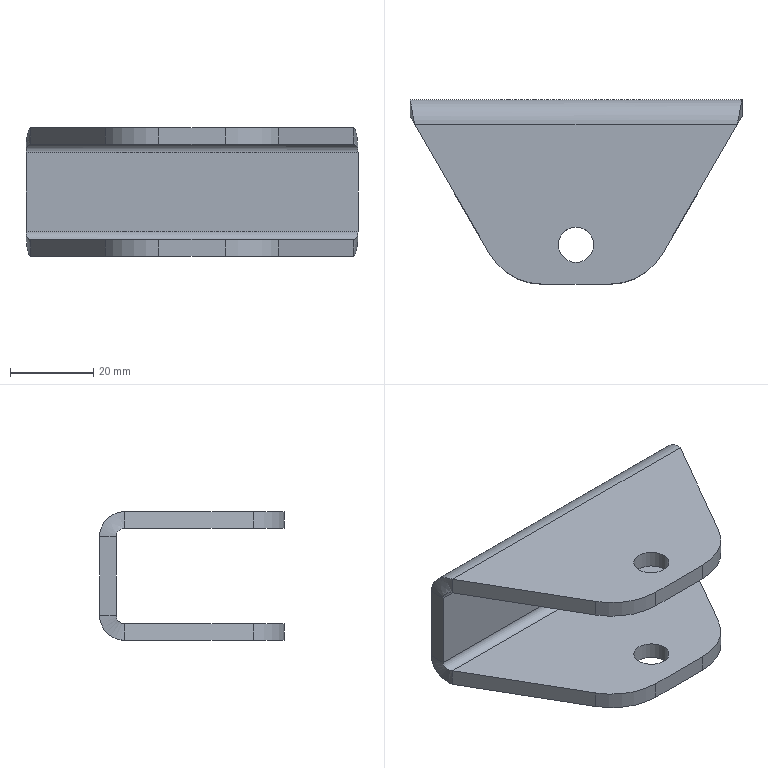Part | STEP file | 6100522 | 1 solid | 28 faces | box 80 x 44.5 x 31 mm | volume 26494 mm3 | plane 14 | cylinder 10 | spline 4 | commonest cylinder face diameters 30 x4 4 x2 8.5 x2 12 x2